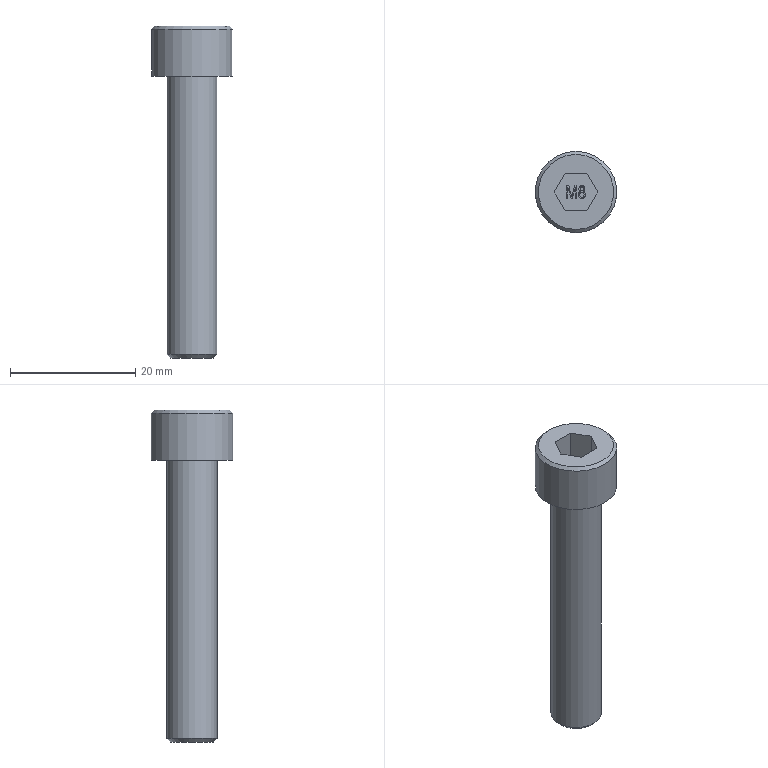Part | STEP file | EM10804500 | 1 solid | 38 faces | box 13 x 13 x 53 mm | volume 3159 mm3 | plane 25 | other 9 | cylinder 2 | cone 2 | commonest cylinder face diameters 8 x1 13 x1